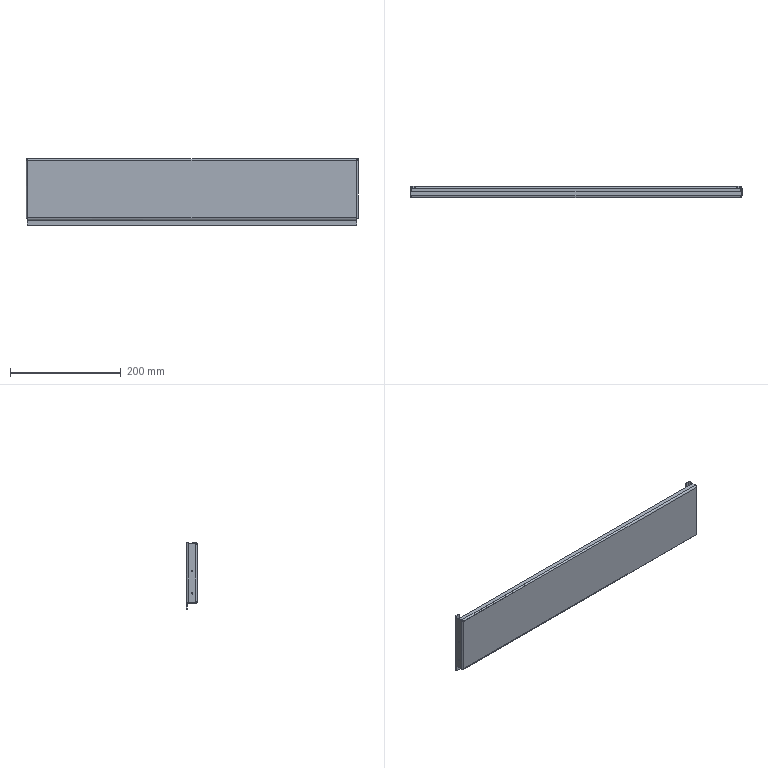Part | STEP file | Sealing plate cover 01001 | 1 solid | 72 faces | box 599 x 20 x 120.5 mm | volume 137683 mm3 | plane 42 | cylinder 22 | spline 8 | commonest cylinder face diameters 2.5 x8 3 x7 6 x7